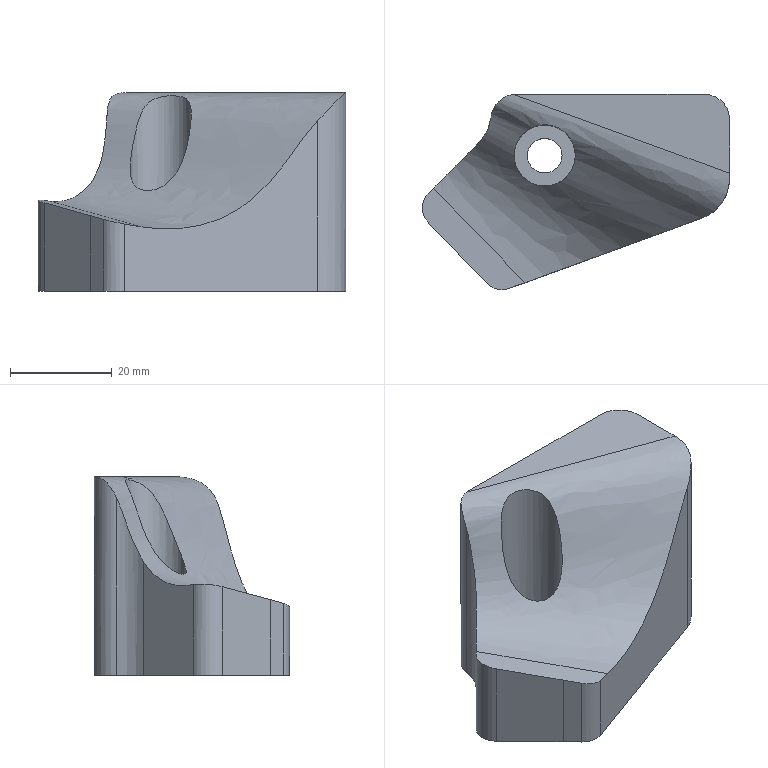Part | STEP file | gslz 2016.10.28-13_id1510_x_t | 1 solid | 19 faces | box 60.365 x 38.336 x 39 mm | volume 43186 mm3 | plane 9 | cylinder 8 | other 1 | spline 1 | commonest cylinder face diameters 8 x2 10 x2 6.8 x1 12 x1 16.6 x1 18 x1